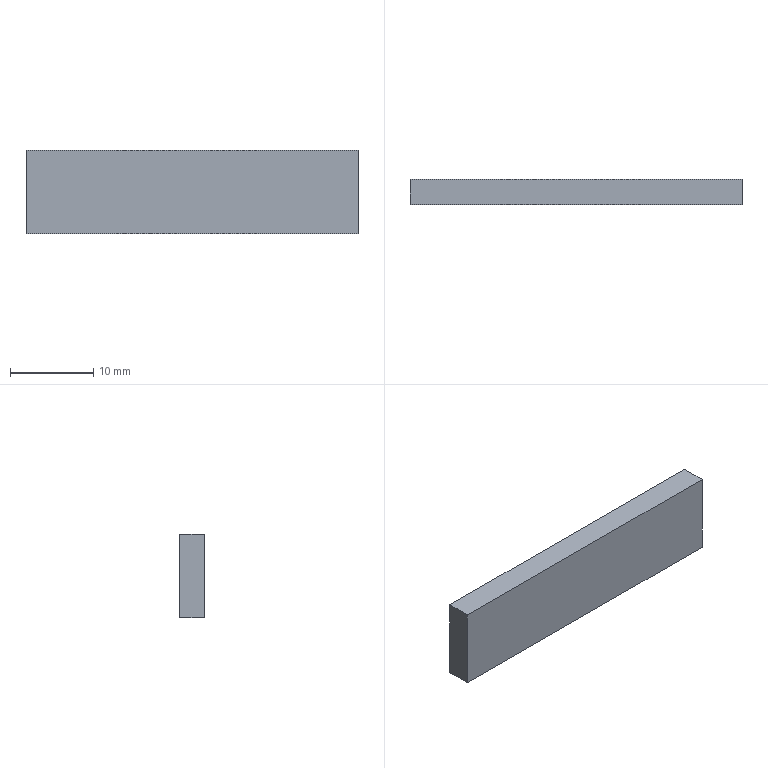Part | STEP file | Guide wheel mechanism revised.sldasm-Part-400 | 1 solid | 6 faces | box 40 x 3 x 10 mm | volume 1200 mm3 | plane 6
STEP:
#1=CARTESIAN_POINT('',(-20.,0.,-20.));
#2=VERTEX_POINT('',#1);
#3=CARTESIAN_POINT('',(-20.,0.,-30.));
#4=VERTEX_POINT('',#3);
#5=CARTESIAN_POINT('',(-20.,0.,-20.));
#6=DIRECTION('',(0.,0.,-1.));
#7=VECTOR('',#6,1000.);
#8=LINE('',#5,#7);
#9=EDGE_CURVE('',#2,#4,#8,.T.);
#10=ORIENTED_EDGE('',*,*,#9,.F.);
#11=CARTESIAN_POINT('',(-20.,3.,-20.));
#12=VERTEX_POINT('',#11);
#13=CARTESIAN_POINT('',(-20.,-41.231,-20.));
#14=DIRECTION('',(0.,1.,0.));
#15=VECTOR('',#14,1000.);
#16=LINE('',#13,#15);
#17=EDGE_CURVE('',#2,#12,#16,.T.);
#18=ORIENTED_EDGE('',*,*,#17,.T.);
#19=CARTESIAN_POINT('',(-20.,3.,-30.));
#20=VERTEX_POINT('',#19);
#21=CARTESIAN_POINT('',(-20.,3.,-20.));
#22=DIRECTION('',(0.,0.,1.));
#23=VECTOR('',#22,1000.);
#24=LINE('',#21,#23);
#25=EDGE_CURVE('',#20,#12,#24,.T.);
#26=ORIENTED_EDGE('',*,*,#25,.F.);
#27=CARTESIAN_POINT('',(-20.,-41.231,-30.));
#28=DIRECTION('',(0.,1.,0.));
#29=VECTOR('',#28,1000.);
#30=LINE('',#27,#29);
#31=EDGE_CURVE('',#4,#20,#30,.T.);
#32=ORIENTED_EDGE('',*,*,#31,.F.);
#33=EDGE_LOOP('',(#10,#18,#26,#32));
#34=FACE_OUTER_BOUND('',#33,.T.);
#35=CARTESIAN_POINT('',(-20.,-41.231,-20.));
#36=DIRECTION('',(-1.,0.,0.));
#37=DIRECTION('',(0.,0.,1.));
#38=AXIS2_PLACEMENT_3D('',#35,#36,#37);
#39=PLANE('',#38);
#40=ADVANCED_FACE('',(#34),#39,.T.);
#41=CARTESIAN_POINT('',(20.,0.,-30.));
#42=VERTEX_POINT('',#41);
#43=CARTESIAN_POINT('',(-20.,0.,-30.));
#44=DIRECTION('',(1.,0.,0.));
#45=VECTOR('',#44,1000.);
#46=LINE('',#43,#45);
#47=EDGE_CURVE('',#4,#42,#46,.T.);
#48=ORIENTED_EDGE('',*,*,#47,.F.);
#49=ORIENTED_EDGE('',*,*,#31,.T.);
#50=CARTESIAN_POINT('',(20.,3.,-30.));
#51=VERTEX_POINT('',#50);
#52=CARTESIAN_POINT('',(-20.,3.,-30.));
#53=DIRECTION('',(-1.,0.,0.));
#54=VECTOR('',#53,1000.);
#55=LINE('',#52,#54);
#56=EDGE_CURVE('',#51,#20,#55,.T.);
#57=ORIENTED_EDGE('',*,*,#56,.F.);
#58=CARTESIAN_POINT('',(20.,-41.231,-30.));
#59=DIRECTION('',(0.,1.,0.));
#60=VECTOR('',#59,1000.);
#61=LINE('',#58,#60);
#62=EDGE_CURVE('',#42,#51,#61,.T.);
#63=ORIENTED_EDGE('',*,*,#62,.F.);
#64=EDGE_LOOP('',(#48,#49,#57,#63));
#65=FACE_OUTER_BOUND('',#64,.T.);
#66=CARTESIAN_POINT('',(-20.,-41.231,-30.));
#67=DIRECTION('',(0.,0.,-1.));
#68=DIRECTION('',(-1.,0.,0.));
#69=AXIS2_PLACEMENT_3D('',#66,#67,#68);
#70=PLANE('',#69);
#71=ADVANCED_FACE('',(#65),#70,.T.);
#72=CARTESIAN_POINT('',(20.,0.,-20.));
#73=VERTEX_POINT('',#72);
#74=CARTESIAN_POINT('',(20.,0.,-20.));
#75=DIRECTION('',(0.,0.,1.));
#76=VECTOR('',#75,1000.);
#77=LINE('',#74,#76);
#78=EDGE_CURVE('',#42,#73,#77,.T.);
#79=ORIENTED_EDGE('',*,*,#78,.F.);
#80=ORIENTED_EDGE('',*,*,#62,.T.);
#81=CARTESIAN_POINT('',(20.,3.,-20.));
#82=VERTEX_POINT('',#81);
#83=CARTESIAN_POINT('',(20.,3.,-20.));
#84=DIRECTION('',(0.,0.,-1.));
#85=VECTOR('',#84,1000.);
#86=LINE('',#83,#85);
#87=EDGE_CURVE('',#82,#51,#86,.T.);
#88=ORIENTED_EDGE('',*,*,#87,.F.);
#89=CARTESIAN_POINT('',(20.,-41.231,-20.));
#90=DIRECTION('',(0.,1.,0.));
#91=VECTOR('',#90,1000.);
#92=LINE('',#89,#91);
#93=EDGE_CURVE('',#73,#82,#92,.T.);
#94=ORIENTED_EDGE('',*,*,#93,.F.);
#95=EDGE_LOOP('',(#79,#80,#88,#94));
#96=FACE_OUTER_BOUND('',#95,.T.);
#97=CARTESIAN_POINT('',(20.,-41.231,-20.));
#98=DIRECTION('',(1.,0.,0.));
#99=DIRECTION('',(0.,0.,-1.));
#100=AXIS2_PLACEMENT_3D('',#97,#98,#99);
#101=PLANE('',#100);
#102=ADVANCED_FACE('',(#96),#101,.T.);
#103=CARTESIAN_POINT('',(-20.,0.,-20.));
#104=DIRECTION('',(-1.,0.,0.));
#105=VECTOR('',#104,1000.);
#106=LINE('',#103,#105);
#107=EDGE_CURVE('',#73,#2,#106,.T.);
#108=ORIENTED_EDGE('',*,*,#107,.F.);
#109=ORIENTED_EDGE('',*,*,#93,.T.);
#110=CARTESIAN_POINT('',(-20.,3.,-20.));
#111=DIRECTION('',(1.,0.,0.));
#112=VECTOR('',#111,1000.);
#113=LINE('',#110,#112);
#114=EDGE_CURVE('',#12,#82,#113,.T.);
#115=ORIENTED_EDGE('',*,*,#114,.F.);
#116=ORIENTED_EDGE('',*,*,#17,.F.);
#117=EDGE_LOOP('',(#108,#109,#115,#116));
#118=FACE_OUTER_BOUND('',#117,.T.);
#119=CARTESIAN_POINT('',(-20.,-41.231,-20.));
#120=DIRECTION('',(0.,0.,1.));
#121=DIRECTION('',(1.,0.,0.));
#122=AXIS2_PLACEMENT_3D('',#119,#120,#121);
#123=PLANE('',#122);
#124=ADVANCED_FACE('',(#118),#123,.T.);
#125=ORIENTED_EDGE('',*,*,#25,.T.);
#126=ORIENTED_EDGE('',*,*,#114,.T.);
#127=ORIENTED_EDGE('',*,*,#87,.T.);
#128=ORIENTED_EDGE('',*,*,#56,.T.);
#129=EDGE_LOOP('',(#125,#126,#127,#128));
#130=FACE_OUTER_BOUND('',#129,.T.);
#131=CARTESIAN_POINT('',(0.,3.,0.));
#132=DIRECTION('',(0.,-1.,0.));
#133=DIRECTION('',(0.,0.,-1.));
#134=AXIS2_PLACEMENT_3D('',#131,#132,#133);
#135=PLANE('',#134);
#136=ADVANCED_FACE('',(#130),#135,.F.);
#137=ORIENTED_EDGE('',*,*,#9,.T.);
#138=ORIENTED_EDGE('',*,*,#47,.T.);
#139=ORIENTED_EDGE('',*,*,#78,.T.);
#140=ORIENTED_EDGE('',*,*,#107,.T.);
#141=EDGE_LOOP('',(#137,#138,#139,#140));
#142=FACE_OUTER_BOUND('',#141,.T.);
#143=CARTESIAN_POINT('',(0.,0.,0.));
#144=DIRECTION('',(0.,1.,0.));
#145=DIRECTION('',(0.,0.,1.));
#146=AXIS2_PLACEMENT_3D('',#143,#144,#145);
#147=PLANE('',#146);
#148=ADVANCED_FACE('',(#142),#147,.F.);
#149=CLOSED_SHELL('',(#40,#71,#102,#124,#136,#148));
#150=MANIFOLD_SOLID_BREP('',#149);
#151=CARTESIAN_POINT('',(0.,0.,0.));
#152=DIRECTION('',(0.,0.,1.));
#153=DIRECTION('',(1.,0.,0.));
#154=AXIS2_PLACEMENT_3D('',#151,#152,#153);
#155=(LENGTH_UNIT()NAMED_UNIT(*)SI_UNIT(.MILLI.,.METRE.));
#156=UNCERTAINTY_MEASURE_WITH_UNIT(LENGTH_MEASURE(0.00001),#155,'','');
#157=(NAMED_UNIT(*)PLANE_ANGLE_UNIT()SI_UNIT($,.RADIAN.));
#158=(NAMED_UNIT(*)SI_UNIT($,.STERADIAN.)SOLID_ANGLE_UNIT());
#159=(GEOMETRIC_REPRESENTATION_CONTEXT(3)GLOBAL_UNCERTAINTY_ASSIGNED_CONTEXT((#156))GLOBAL_UNIT_ASSIGNED_CONTEXT((#155,#157,#158))REPRESENTATION_CONTEXT('',''));
#160=ADVANCED_BREP_SHAPE_REPRESENTATION('',(#150,#154),#159);